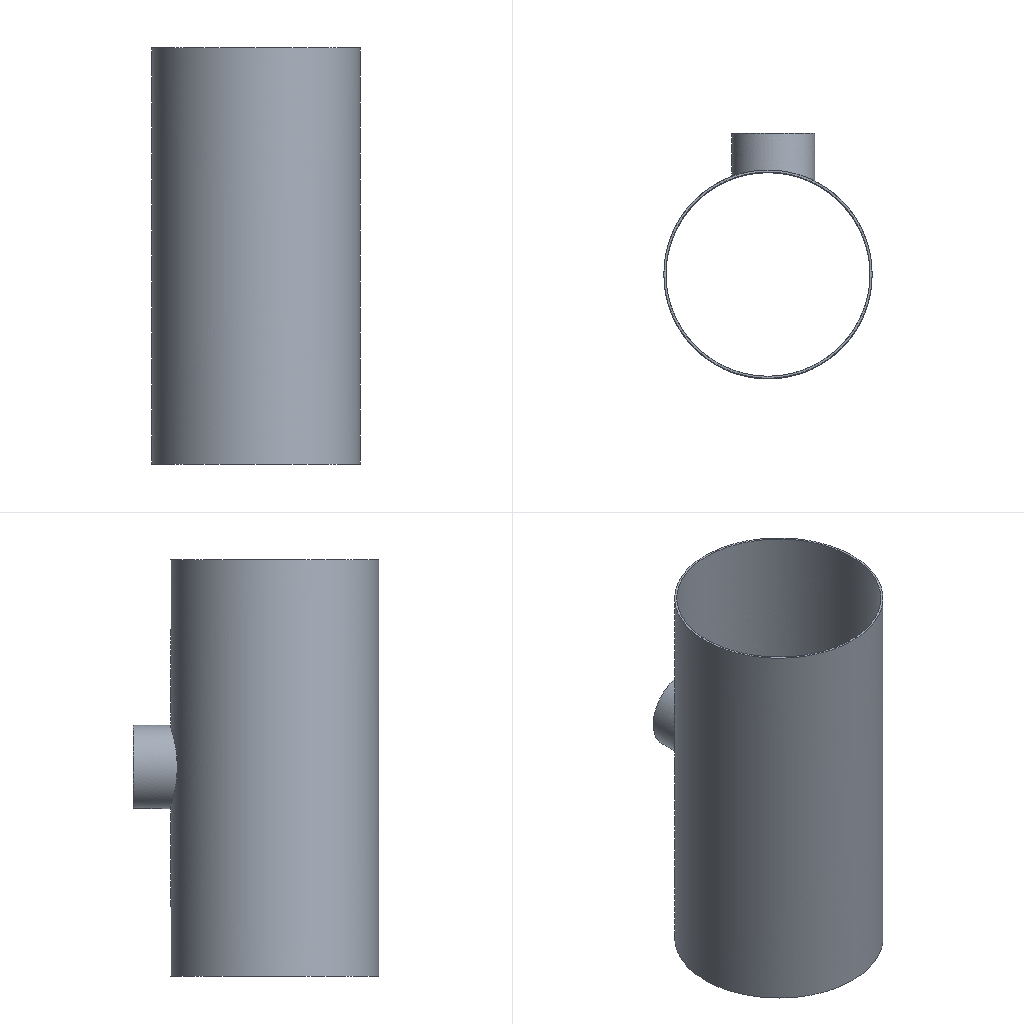Simulation study | ansys workbench
Set-up summary:
category,name,step,type,value,unit,region
solver,ansys_workbench
units,mm-N-s-tonne (MPa),,stated,"/units,MPA"
analysis,LS1,,static
load_step,LS1,LS1,static,nsubst=1; time=1
mesh,nodes,,,232772
mesh,elements,,,154573
element_type,SOLID187,,,117565
element_type,SURF154,,,37008
material,Structural Steel,,E,200000,tonne s^-2 mm^-1
material,Structural Steel,,nu,0.3
material,Structural Steel,,density,7.85e-09,tonne mm^-3
material,Structural Steel,,conductivity,60.5,tonne mm s^-3 C^-1
material,Structural Steel,,specific_heat,4.34e+08,mm^2 s^-2 C^-1
material,Structural Steel,,cte,1.2e-05,C^-1
material,Structural Steel,,permeability,10000
material,Structural Steel,,resistivity,0.00017,ohm mm
load,"Define Pressure Using Surface Effect Elements ""__""",LS1,pressure,5e-05,,SURF154 #2
bc,Fixed Supports,model,fixed,[dofs=ALL],,_FIXEDSU
named_set,_FIXEDSU,,node,1872
Ansys APDL input file, long lists of numbers shortened:
/batch
/config,noeldb,1     ! force off writing results to database
*get,_wallstrt,active,,time,wall
! ANSYS input file written by Workbench version 2024 R2
! File used for geometry attach:
/title,wbnew--____ (A5)
! ****** Begin Custom Load Command Snippet ******
/COM, ACT Extensions:
/COM,     LSDYNA, 2024.2
/COM,/COM,     ANSYSMotion, 2024.2
/COM,
! ****** End   Custom Load Command Snippet ******
*DIM,_wb_ProjectScratch_dir,string,248
_wb_ProjectScratch_dir(1) = ''
*DIM,_wb_SolverFiles_dir,string,248
_wb_SolverFiles_dir(1) = ''
*DIM,_wb_userfiles_dir,string,248
_wb_userfiles_dir(1) = ''
/com,--- Data in consistent NMM units. See Solving Units in the help system for more information.
/units,MPA
/nopr
/wb,file,start              !  signify a WB generated input file
/prep7
! Turn off shape checking because checks already performed inside WB mesher.
! See help system for more information.
SHPP,OFF,,NOWARN
/nolist
etcon,set             ! allow ANSYS to choose best KEYOP's for 180x elements, resets any applicable keyopt to MAPDL defaults
/com,*********** Nodes for the whole assembly ***********
nblock,3,,256049
(1i9,3e20.9e3)
        1    -1.451294788E+02     5.224248460E+02     8.826152273E+02
! (232771 more lines like these left out)
-1
/wb,elem,start            !  set before creation of elements
/com,*********** Elements for Body 1 '____-FreeParts|__-__3' ***********
et,1,187
eblock,19,solid,,117565
(19i9)
        1        1        1        1        0        0        0        0       10        0        1    19900    20478    38666    19901   142758   232748   232745   140343
! (235129 more lines like these left out)
-1
/wb,elem,end               !  done creating elements
/com,*********** Send User Defined Coordinate System(s) ***********
csys,0
toffst,273.15,      ! Temperature offset from absolute zero
/com,*********** Set Reference Temperature ***********
tref,22.
/wb,mat,start              !  starting to send materials
/com,*********** Send Materials ***********
Temperature = 'TEMP' ! Temperature
MP,DENS,1,7.85e-09,	! tonne mm^-3
MP,ALPX,1,1.2e-05,	! C^-1
MP,C,1,434000000,	! mm^2 s^-2 C^-1
MP,KXX,1,60.5,	! tonne mm s^-3 C^-1
MP,RSVX,1,0.00017,	! ohm mm
MP,EX,1,200000,	! tonne s^-2 mm^-1
MP,NUXY,1,0.3,
MP,MURX,1,10000,
/wb,mat,end                !  done sending materials
!************************* Model Summary ********************
!压力容器-FreeParts|切除-拉伸3,	结构钢,	matid,	1
!************************* End Model Summary ********************
! get the diagonal of the bounding box. Needed later for other things
*get,_xmin,node,,mnloc,x
*get,_ymin,node,,mnloc,y
*get,_zmin,node,,mnloc,z
*get,_xmax,node,,mxloc,x
*get,_ymax,node,,mxloc,y
*get,_zmax,node,,mxloc,z
_ASMDIAG=(_xmax-_xmin)*(_xmax-_xmin)+(_ymax-_ymin)*(_ymax-_ymin)+(_zmax-_zmin)*(_zmax-_zmin)
_ASMDIAG=SQRT(_ASMDIAG)
/wb,contact,start          !  starting to send contact
/wb,contact,end            !  done creating contacts
/golist
/wb,load,start             !  starting to send loads
/com,*********** Fixed Supports ***********
CMBLOCK,_FIXEDSU,NODE,     1872
(8i10)
     37489     37490     37491     37492     37493     37494     37495     37496
! (233 more lines like these left out)
cmsel,s,_FIXEDSU
d,all,all
nsel,all
/com,*********** Define Pressure Using Surface Effect Elements "__" ***********
et,2,154
mat,2
eblock,10,,,37008
(15i9)
   193170        2        2        2        0    30373    30085    30372    30372   177155   177149    30372   177157
! (37007 more lines like these left out)
-1
esel,s,type,,2
keyop,2,7,0         ! Use deformed area for application of load
esel,all
esel,all
/gst,on,on
fini
*get,_numnode,node,0,count
*get,_numelem,elem,0,count
*get, _MAXELEMNUM, elem, 0, NUM, MAX
*get, _MAXNODENUM, node, 0, NUM, MAX
*get, _MAXELEMTYPE, etyp, 0, NUM, MAX
*get, _MAXREALCONST, rcon, 0, NUM, MAX
/go
/wb,load,end               !  done creating loads
/com,--- Number of total nodes = %_numnode%
/com,--- Number of contact elements = 37008
/com,--- Number of spring elements = 0
/com,--- Number of bearing elements = 0
/com,--- Number of solid elements = 117565
/com,--- Number of condensed parts = 0
/com,--- Number of total elements = %_numelem%
*get,_wallbsol,active,,time,wall
/com,****************************************************************************
/com,*************************    SOLUTION       ********************************
/com,****************************************************************************
/solu
antype,0                   ! static analysis
_thickRatio=  1     ! Ratio of thick parts in the model
eqsl,pcg,1e-8,,,,,,1
cntr,print,1               ! print out contact info and also make no initial contact an error
cncheck,dmp		!	Enable program controlled contact splitting for distributed memory parallel run
dmpoption,emat,no             ! Don't combine emat file for DANSYS
dmpoption,esav,no             ! Don't combine esav file for DANSYS
nldiag,cont,iter           ! print out contact info each equilibrium iteration
rescontrol,,none                 ! Do not keep any restart files
/com,****************************************************
/com,******************* SOLVE FOR LS 1 OF 1 ****************
esel,s,type,,2
nsle
sf,all,pres,5.e-005
nsel,all
esel,all
esel,all
/nopr
/gopr
nsub,1,1,1
time,1.
outres,erase
outres,all,none
outres,nsol,all,
outres,rsol,all
outres,eangl,all
outres,etmp,all
outres,veng,all
outres,strs,all,
outres,epel,all,
outres,eppl,all,
outres,cont,all,
! *********** WB SOLVE COMMAND ***********
! check interactive state
*get,ANSINTER_,active,,int
*if,ANSINTER_,ne,0,then
/eof
*endif
solve
/com *************** Write FE CONNECTORS *********
CEWRITE,file,ce,,INTE
/com,****************************************************
/com,*************** FINISHED SOLVE FOR LS 1 *************
*get,_wallasol,active,,time,wall
/nopr
*get,_numnode,node,0,count
*get,_numelem,elem,0,count
*get, _MAXELEMNUM, elem, 0, NUM, MAX
*get, _MAXNODENUM, node, 0, NUM, MAX,,,INTERNAL
*get, _MAXELEMTYPE, etyp, 0, NUM, MAX
*get, _MAXREALCONST, rcon, 0, NUM, MAX
*get,_NSOLTHREADS,active,0,ntfs
*get,_NSOLPROCESSES,active,0,npfs
/gopr
*get,_PCGITER,active,,solu,cgiter
/post1
xmlo,ENCODING,ISO-8859-1
xmlo,parm
/xml,parm,xml
fini
/gopr
*get,_walldone,active,,time,wall
_preptime=(_wallbsol-_wallstrt)*3600
_solvtime=(_wallasol-_wallbsol)*3600
_posttime=(_walldone-_wallasol)*3600
_totaltim=(_walldone-_wallstrt)*3600
*get,_dlbratio,active,0,solu,dlbr
*get,_combtime,active,0,solu,comb
*get,_ssmode,active,0,solu,ssmm
*get,_ndofs,active,0,solu,ndof
*get,_sol_end_time,active,0,set,time
*if,_sol_end_time,eq,1.,then
/fclean				!clean distributed files
*endif
/com,--- Total number of nodes = %_numnode%
/com,--- Total number of elements = %_numelem%
/com,--- Element load balance ratio = %_dlbratio%
/com,--- Time to combine distributed files = %_combtime%
/com,--- Sparse memory mode = %_ssmode%
/com,--- Number of DOF = %_ndofs%
/wb,file,end               ! done with WB generated input
Results summary:
result,analyses[0].index,,,1
result,analyses[0].system,,,SYS
result,analyses[0].deck,,,deck.dat
result,analyses[0].solve_status,,,completed
result,analyses[0].analysis_type,,,static
result,analyses[0].physics,,,mechanical
result,analyses[0].unit_system,,,"NMM: mm, ton, N, s, mV, mA, degC"
result,analyses[0].n_sets,,,1
result,analyses[0].load_steps[0].set,set=1,,1
result,analyses[0].load_steps[0].time_or_freq,set=1,,1
result,analyses[0].load_steps[0].max_displacement_magnitude,set=1,,9.56526e-05
result,analyses[0].load_steps[0].max_von_mises_nodal,set=1,,0.01306
result,analyses[0].load_steps[0].reaction_force_sum_xyz[1],set=1,,1.12888e-08
result,analyses[0].load_steps[0].reaction_force_sum_xyz[2],set=1,,5.671
result,analyses[0].load_steps[0].reaction_force_sum_xyz[3],set=1,,-4.40952e-09